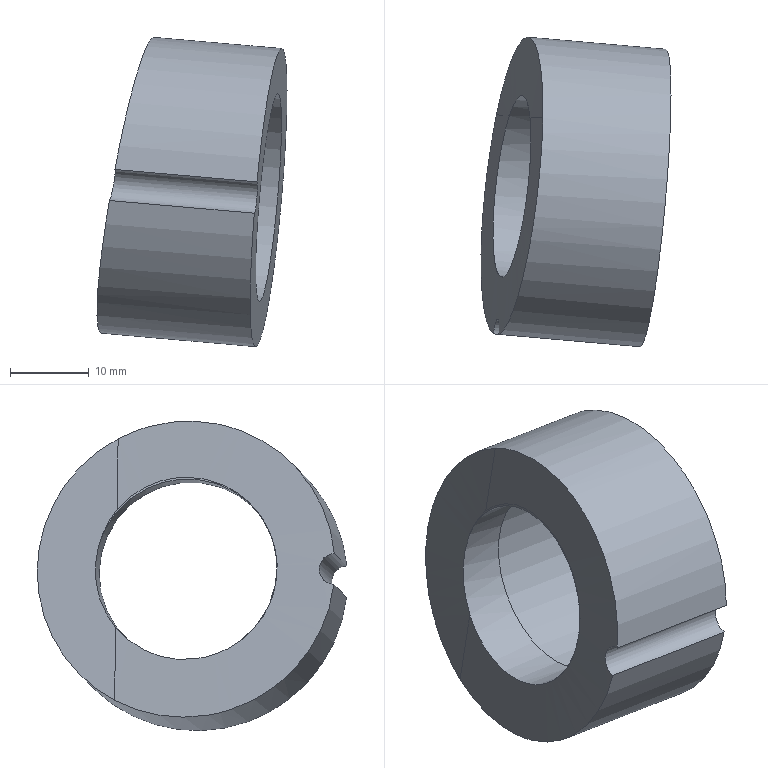Part | NX | features solid 2 | 1 solid | 10 faces | box 24.121 x 39.295 x 39.277 mm | volume 11087 mm3 | cylinder 4 | spline 4 | plane 2 | commonest cylinder face diameters 4 x1 23.2 x1 26.6 x1 38 x1
STEP:
#1=CARTESIAN_POINT('',(-929.483,-260.051,-35.553));
#2=VERTEX_POINT('',#1);
#3=CARTESIAN_POINT('',(-923.901,-232.605,-21.002));
#4=VERTEX_POINT('',#3);
#5=CARTESIAN_POINT('',(-929.483,-260.051,-35.553));
#6=CARTESIAN_POINT('',(-928.909,-259.773,-32.489));
#7=CARTESIAN_POINT('',(-927.663,-257.698,-26.623));
#8=CARTESIAN_POINT('',(-925.814,-250.756,-20.295));
#9=CARTESIAN_POINT('',(-924.374,-241.535,-18.016));
#10=CARTESIAN_POINT('',(-923.946,-235.373,-19.542));
#11=CARTESIAN_POINT('',(-923.901,-232.605,-21.002));
#12=B_SPLINE_CURVE_WITH_KNOTS('',3,(#5,#6,#7,#8,#9,#10,#11),.UNSPECIFIED.,.F.,.F.,(4,1,1,1,4),(0.,0.009255,0.01851,0.02776,0.03702),.UNSPECIFIED.);
#13=EDGE_CURVE('',#2,#4,#12,.T.);
#14=ORIENTED_EDGE('',*,*,#13,.F.);
#15=CARTESIAN_POINT('',(-911.448,-261.629,-37.137));
#16=VERTEX_POINT('',#15);
#17=CARTESIAN_POINT('',(-921.372,-260.761,-36.265));
#18=DIRECTION('',(-0.9924,0.08682,0.08716));
#19=VECTOR('',#18,1000.);
#20=LINE('',#17,#19);
#21=EDGE_CURVE('',#16,#2,#20,.T.);
#22=ORIENTED_EDGE('',*,*,#21,.F.);
#23=CARTESIAN_POINT('',(-911.795,-261.599,-41.116));
#24=VERTEX_POINT('',#23);
#25=CARTESIAN_POINT('',(-909.974,-242.791,-39.126));
#26=DIRECTION('',(-0.9924,0.08682,0.08716));
#27=DIRECTION('',(-0.08716,-0.9962,0.));
#28=AXIS2_PLACEMENT_3D('',#25,#26,#27);
#29=CIRCLE('',#28,19.);
#30=EDGE_CURVE('',#16,#24,#29,.T.);
#31=ORIENTED_EDGE('',*,*,#30,.T.);
#32=CARTESIAN_POINT('',(-930.183,-259.99,-39.501));
#33=VERTEX_POINT('',#32);
#34=CARTESIAN_POINT('',(-921.719,-260.731,-40.244));
#35=DIRECTION('',(-0.9924,0.08682,0.08716));
#36=VECTOR('',#35,1000.);
#37=LINE('',#34,#36);
#38=EDGE_CURVE('',#33,#24,#37,.F.);
#39=ORIENTED_EDGE('',*,*,#38,.F.);
#40=CARTESIAN_POINT('',(-929.786,-232.163,-54.19));
#41=VERTEX_POINT('',#40);
#42=CARTESIAN_POINT('',(-929.786,-232.163,-54.19));
#43=CARTESIAN_POINT('',(-930.342,-234.88,-55.62));
#44=CARTESIAN_POINT('',(-931.297,-240.963,-57.09));
#45=CARTESIAN_POINT('',(-931.921,-250.215,-54.784));
#46=CARTESIAN_POINT('',(-931.526,-257.369,-48.427));
#47=CARTESIAN_POINT('',(-930.693,-259.618,-42.557));
#48=CARTESIAN_POINT('',(-930.183,-259.99,-39.501));
#49=B_SPLINE_CURVE_WITH_KNOTS('',3,(#42,#43,#44,#45,#46,#47,#48),.UNSPECIFIED.,.F.,.F.,(4,1,1,1,4),(0.,0.00923,0.01846,0.02769,0.03692),.UNSPECIFIED.);
#50=EDGE_CURVE('',#41,#33,#49,.T.);
#51=ORIENTED_EDGE('',*,*,#50,.F.);
#52=CARTESIAN_POINT('',(-923.901,-232.605,-21.002));
#53=CARTESIAN_POINT('',(-923.851,-229.534,-22.621));
#54=CARTESIAN_POINT('',(-924.167,-224.375,-27.458));
#55=CARTESIAN_POINT('',(-925.684,-221.388,-37.657));
#56=CARTESIAN_POINT('',(-927.766,-224.091,-47.767));
#57=CARTESIAN_POINT('',(-929.167,-229.14,-52.598));
#58=CARTESIAN_POINT('',(-929.786,-232.163,-54.19));
#59=B_SPLINE_CURVE_WITH_KNOTS('',3,(#52,#53,#54,#55,#56,#57,#58),.UNSPECIFIED.,.F.,.F.,(4,1,1,1,4),(0.,0.01027,0.02053,0.0308,0.04107),.UNSPECIFIED.);
#60=EDGE_CURVE('',#4,#41,#59,.T.);
#61=ORIENTED_EDGE('',*,*,#60,.F.);
#62=EDGE_LOOP('',(#14,#22,#31,#39,#51,#61));
#63=FACE_BOUND('',#62,.T.);
#64=CARTESIAN_POINT('',(-909.974,-242.791,-39.126));
#65=DIRECTION('',(-0.9924,0.08682,0.08716));
#66=DIRECTION('',(-0.08716,-0.9962,0.));
#67=AXIS2_PLACEMENT_3D('',#64,#65,#66);
#68=CYLINDRICAL_SURFACE('',#67,19.);
#69=ADVANCED_FACE('',(#63),#68,.T.);
#70=CARTESIAN_POINT('',(-911.134,-256.041,-39.126));
#71=VERTEX_POINT('',#70);
#72=CARTESIAN_POINT('',(-909.974,-242.791,-39.126));
#73=DIRECTION('',(-0.9924,0.08682,0.08716));
#74=DIRECTION('',(-0.08716,-0.9962,0.));
#75=AXIS2_PLACEMENT_3D('',#72,#73,#74);
#76=CIRCLE('',#75,13.3);
#77=EDGE_CURVE('',#71,#71,#76,.T.);
#78=ORIENTED_EDGE('',*,*,#77,.T.);
#79=EDGE_LOOP('',(#78));
#80=FACE_BOUND('',#79,.T.);
#81=ORIENTED_EDGE('',*,*,#30,.F.);
#82=CARTESIAN_POINT('',(-911.63,-261.719,-39.126));
#83=DIRECTION('',(-0.9924,0.08682,0.08716));
#84=DIRECTION('',(-0.08716,-0.9962,0.));
#85=AXIS2_PLACEMENT_3D('',#82,#83,#84);
#86=CIRCLE('',#85,2.);
#87=EDGE_CURVE('',#16,#24,#86,.T.);
#88=ORIENTED_EDGE('',*,*,#87,.T.);
#89=EDGE_LOOP('',(#81,#88));
#90=FACE_BOUND('',#89,.T.);
#91=CARTESIAN_POINT('',(-909.974,-242.791,-39.126));
#92=DIRECTION('',(-0.9924,0.08682,0.08716));
#93=DIRECTION('',(-0.08716,-0.9962,0.));
#94=AXIS2_PLACEMENT_3D('',#91,#92,#93);
#95=PLANE('',#94);
#96=ADVANCED_FACE('',(#80,#90),#95,.F.);
#97=ORIENTED_EDGE('',*,*,#77,.F.);
#98=EDGE_LOOP('',(#97));
#99=FACE_BOUND('',#98,.T.);
#100=CARTESIAN_POINT('',(-923.042,-254.999,-38.08));
#101=VERTEX_POINT('',#100);
#102=CARTESIAN_POINT('',(-921.883,-241.749,-38.08));
#103=DIRECTION('',(-0.9924,0.08682,0.08716));
#104=DIRECTION('',(-0.08716,-0.9962,0.));
#105=AXIS2_PLACEMENT_3D('',#102,#103,#104);
#106=CIRCLE('',#105,13.3);
#107=EDGE_CURVE('',#101,#101,#106,.T.);
#108=ORIENTED_EDGE('',*,*,#107,.T.);
#109=EDGE_LOOP('',(#108));
#110=FACE_BOUND('',#109,.T.);
#111=CARTESIAN_POINT('',(-909.974,-242.791,-39.126));
#112=DIRECTION('',(-0.9924,0.08682,0.08716));
#113=DIRECTION('',(-0.08716,-0.9962,0.));
#114=AXIS2_PLACEMENT_3D('',#111,#112,#113);
#115=CYLINDRICAL_SURFACE('',#114,13.3);
#116=ADVANCED_FACE('',(#99,#110),#115,.F.);
#117=CARTESIAN_POINT('',(-922.894,-253.305,-38.08));
#118=VERTEX_POINT('',#117);
#119=CARTESIAN_POINT('',(-921.883,-241.749,-38.08));
#120=DIRECTION('',(-0.9924,0.08682,0.08716));
#121=DIRECTION('',(-0.08716,-0.9962,0.));
#122=AXIS2_PLACEMENT_3D('',#119,#120,#121);
#123=CIRCLE('',#122,11.6);
#124=EDGE_CURVE('',#118,#118,#123,.T.);
#125=ORIENTED_EDGE('',*,*,#124,.T.);
#126=EDGE_LOOP('',(#125));
#127=FACE_BOUND('',#126,.T.);
#128=ORIENTED_EDGE('',*,*,#107,.F.);
#129=EDGE_LOOP('',(#128));
#130=FACE_BOUND('',#129,.T.);
#131=CARTESIAN_POINT('',(-921.883,-241.749,-38.08));
#132=DIRECTION('',(-0.9924,0.08682,0.08716));
#133=DIRECTION('',(-0.08716,-0.9962,0.));
#134=AXIS2_PLACEMENT_3D('',#131,#132,#133);
#135=PLANE('',#134);
#136=ADVANCED_FACE('',(#127,#130),#135,.F.);
#137=ORIENTED_EDGE('',*,*,#21,.T.);
#138=CARTESIAN_POINT('',(-929.483,-260.051,-35.553));
#139=CARTESIAN_POINT('',(-929.439,-259.542,-35.58));
#140=CARTESIAN_POINT('',(-929.424,-258.559,-36.034));
#141=CARTESIAN_POINT('',(-929.629,-257.934,-37.53));
#142=CARTESIAN_POINT('',(-929.954,-258.513,-39.023));
#143=CARTESIAN_POINT('',(-930.129,-259.482,-39.475));
#144=CARTESIAN_POINT('',(-930.183,-259.99,-39.501));
#145=B_SPLINE_CURVE_WITH_KNOTS('',3,(#138,#139,#140,#141,#142,#143,#144),.UNSPECIFIED.,.F.,.F.,(4,1,1,1,4),(0.,0.001514,0.003028,0.004542,0.006057),.UNSPECIFIED.);
#146=EDGE_CURVE('',#2,#33,#145,.T.);
#147=ORIENTED_EDGE('',*,*,#146,.T.);
#148=ORIENTED_EDGE('',*,*,#38,.T.);
#149=ORIENTED_EDGE('',*,*,#87,.F.);
#150=EDGE_LOOP('',(#137,#147,#148,#149));
#151=FACE_BOUND('',#150,.T.);
#152=CARTESIAN_POINT('',(-911.63,-261.719,-39.126));
#153=DIRECTION('',(-0.9924,0.08682,0.08716));
#154=DIRECTION('',(-0.08716,-0.9962,0.));
#155=AXIS2_PLACEMENT_3D('',#152,#153,#154);
#156=CYLINDRICAL_SURFACE('',#155,2.);
#157=ADVANCED_FACE('',(#151),#156,.F.);
#158=CARTESIAN_POINT('',(-926.06,-230.143,-34.59));
#159=VERTEX_POINT('',#158);
#160=CARTESIAN_POINT('',(-925.539,-232.482,-30.239));
#161=VERTEX_POINT('',#160);
#162=CARTESIAN_POINT('',(-926.06,-230.143,-34.59));
#163=CARTESIAN_POINT('',(-925.828,-230.596,-33.013));
#164=CARTESIAN_POINT('',(-925.647,-231.395,-31.516));
#165=CARTESIAN_POINT('',(-925.539,-232.482,-30.239));
#166=B_SPLINE_CURVE_WITH_KNOTS('',3,(#162,#163,#164,#165),.UNSPECIFIED.,.F.,.F.,(4,4),(0.001876,0.006846),.UNSPECIFIED.);
#167=EDGE_CURVE('',#159,#161,#166,.T.);
#168=ORIENTED_EDGE('',*,*,#167,.F.);
#169=CARTESIAN_POINT('',(-928.148,-232.286,-44.953));
#170=VERTEX_POINT('',#169);
#171=CARTESIAN_POINT('',(-926.06,-230.143,-34.59));
#172=CARTESIAN_POINT('',(-926.584,-229.124,-38.139));
#173=CARTESIAN_POINT('',(-927.379,-229.926,-42.112));
#174=CARTESIAN_POINT('',(-928.148,-232.286,-44.953));
#175=B_SPLINE_CURVE_WITH_KNOTS('',3,(#171,#172,#173,#174),.UNSPECIFIED.,.F.,.F.,(4,4),(0.004979,0.01613),.UNSPECIFIED.);
#176=EDGE_CURVE('',#159,#170,#175,.T.);
#177=ORIENTED_EDGE('',*,*,#176,.T.);
#178=CARTESIAN_POINT('',(-930.229,-247.913,-46.785));
#179=VERTEX_POINT('',#178);
#180=CARTESIAN_POINT('',(-928.148,-232.286,-44.953));
#181=CARTESIAN_POINT('',(-928.747,-234.127,-47.168));
#182=CARTESIAN_POINT('',(-929.874,-239.507,-50.064));
#183=CARTESIAN_POINT('',(-930.275,-245.564,-48.485));
#184=CARTESIAN_POINT('',(-930.229,-247.913,-46.785));
#185=B_SPLINE_CURVE_WITH_KNOTS('',3,(#180,#181,#182,#183,#184),.UNSPECIFIED.,.F.,.F.,(4,1,4),(0.,0.0087,0.0174),.UNSPECIFIED.);
#186=EDGE_CURVE('',#170,#179,#185,.T.);
#187=ORIENTED_EDGE('',*,*,#186,.T.);
#188=CARTESIAN_POINT('',(-925.539,-232.482,-30.239));
#189=CARTESIAN_POINT('',(-925.326,-234.624,-27.725));
#190=CARTESIAN_POINT('',(-925.507,-241.044,-24.655));
#191=CARTESIAN_POINT('',(-927.325,-250.854,-28.707));
#192=CARTESIAN_POINT('',(-929.453,-254.13,-38.716));
#193=CARTESIAN_POINT('',(-930.177,-250.588,-44.848));
#194=CARTESIAN_POINT('',(-930.229,-247.913,-46.785));
#195=B_SPLINE_CURVE_WITH_KNOTS('',3,(#188,#189,#190,#191,#192,#193,#194),.UNSPECIFIED.,.F.,.F.,(4,1,1,1,4),(0.,0.009788,0.01958,0.02936,0.03915),.UNSPECIFIED.);
#196=EDGE_CURVE('',#161,#179,#195,.T.);
#197=ORIENTED_EDGE('',*,*,#196,.F.);
#198=EDGE_LOOP('',(#168,#177,#187,#197));
#199=FACE_BOUND('',#198,.T.);
#200=ORIENTED_EDGE('',*,*,#124,.F.);
#201=EDGE_LOOP('',(#200));
#202=FACE_BOUND('',#201,.T.);
#203=CARTESIAN_POINT('',(-909.974,-242.791,-39.126));
#204=DIRECTION('',(-0.9924,0.08682,0.08716));
#205=DIRECTION('',(-0.08716,-0.9962,0.));
#206=AXIS2_PLACEMENT_3D('',#203,#204,#205);
#207=CYLINDRICAL_SURFACE('',#206,11.6);
#208=ADVANCED_FACE('',(#199,#202),#207,.F.);
#209=CARTESIAN_POINT('',(-925.496,-232.485,-29.998));
#210=VERTEX_POINT('',#209);
#211=CARTESIAN_POINT('',(-925.496,-232.485,-29.998));
#212=CARTESIAN_POINT('',(-924.965,-232.525,-26.999));
#213=CARTESIAN_POINT('',(-924.433,-232.565,-24.001));
#214=CARTESIAN_POINT('',(-923.901,-232.605,-21.002));
#215=B_SPLINE_CURVE_WITH_KNOTS('',3,(#211,#212,#213,#214),.UNSPECIFIED.,.F.,.F.,(4,4),(0.,0.6033),.UNSPECIFIED.);
#216=EDGE_CURVE('',#210,#4,#215,.T.);
#217=ORIENTED_EDGE('',*,*,#216,.T.);
#218=ORIENTED_EDGE('',*,*,#60,.T.);
#219=CARTESIAN_POINT('',(-929.786,-232.163,-54.19));
#220=CARTESIAN_POINT('',(-929.24,-232.204,-51.111));
#221=CARTESIAN_POINT('',(-928.694,-232.245,-48.032));
#222=CARTESIAN_POINT('',(-928.148,-232.286,-44.953));
#223=B_SPLINE_CURVE_WITH_KNOTS('',3,(#219,#220,#221,#222),.UNSPECIFIED.,.F.,.F.,(4,4),(0.3603,0.9722),.UNSPECIFIED.);
#224=EDGE_CURVE('',#41,#170,#223,.T.);
#225=ORIENTED_EDGE('',*,*,#224,.T.);
#226=ORIENTED_EDGE('',*,*,#176,.F.);
#227=CARTESIAN_POINT('',(-926.06,-230.143,-34.59));
#228=CARTESIAN_POINT('',(-925.813,-230.555,-32.954));
#229=CARTESIAN_POINT('',(-925.613,-231.354,-31.348));
#230=CARTESIAN_POINT('',(-925.496,-232.485,-29.998));
#231=B_SPLINE_CURVE_WITH_KNOTS('',3,(#227,#228,#229,#230),.UNSPECIFIED.,.F.,.F.,(4,4),(0.6832,1.),.UNSPECIFIED.);
#232=EDGE_CURVE('',#159,#210,#231,.T.);
#233=ORIENTED_EDGE('',*,*,#232,.T.);
#234=EDGE_LOOP('',(#217,#218,#225,#226,#233));
#235=FACE_BOUND('',#234,.T.);
#236=CARTESIAN_POINT('',(-929.075,-221.938,-56.328));
#237=CARTESIAN_POINT('',(-923.118,-222.354,-22.742));
#238=CARTESIAN_POINT('',(-929.22,-223.985,-55.955));
#239=CARTESIAN_POINT('',(-923.263,-224.408,-22.369));
#240=CARTESIAN_POINT('',(-929.367,-226.031,-55.575));
#241=CARTESIAN_POINT('',(-923.41,-226.46,-21.989));
#242=CARTESIAN_POINT('',(-929.516,-228.076,-55.188));
#243=CARTESIAN_POINT('',(-923.56,-228.511,-21.602));
#244=CARTESIAN_POINT('',(-929.667,-230.119,-54.792));
#245=CARTESIAN_POINT('',(-923.712,-230.56,-21.206));
#246=CARTESIAN_POINT('',(-929.821,-232.16,-54.389));
#247=CARTESIAN_POINT('',(-923.866,-232.608,-20.803));
#248=B_SPLINE_SURFACE_WITH_KNOTS('',5,1,((#236,#237),(#238,#239),(#240,#241),(#242,#243),(#244,#245),(#246,#247)),.RULED_SURF.,.F.,.F.,.F.,(6,6),(2,2),(0.9701,1.),(0.1222,0.8673),.PIECEWISE_BEZIER_KNOTS.);
#249=ADVANCED_FACE('',(#235),#248,.T.);
#250=ORIENTED_EDGE('',*,*,#146,.F.);
#251=ORIENTED_EDGE('',*,*,#13,.T.);
#252=ORIENTED_EDGE('',*,*,#216,.F.);
#253=CARTESIAN_POINT('',(-925.752,-241.299,-25.884));
#254=VERTEX_POINT('',#253);
#255=CARTESIAN_POINT('',(-925.496,-232.485,-29.998));
#256=CARTESIAN_POINT('',(-925.439,-233.04,-29.336));
#257=CARTESIAN_POINT('',(-925.365,-234.254,-28.166));
#258=CARTESIAN_POINT('',(-925.384,-237.251,-26.392));
#259=CARTESIAN_POINT('',(-925.562,-239.62,-25.884));
#260=CARTESIAN_POINT('',(-925.752,-241.299,-25.884));
#261=B_SPLINE_CURVE_WITH_KNOTS('',3,(#255,#256,#257,#258,#259,#260),.UNSPECIFIED.,.F.,.F.,(4,1,1,4),(0.,0.25,0.5,1.),.UNSPECIFIED.);
#262=EDGE_CURVE('',#210,#254,#261,.T.);
#263=ORIENTED_EDGE('',*,*,#262,.T.);
#264=CARTESIAN_POINT('',(-929.986,-251.003,-43.546));
#265=VERTEX_POINT('',#264);
#266=CARTESIAN_POINT('',(-925.752,-241.299,-25.884));
#267=CARTESIAN_POINT('',(-925.983,-243.35,-25.883));
#268=CARTESIAN_POINT('',(-926.635,-247.369,-27.));
#269=CARTESIAN_POINT('',(-927.88,-251.708,-31.336));
#270=CARTESIAN_POINT('',(-928.941,-253.09,-36.457));
#271=CARTESIAN_POINT('',(-929.622,-252.482,-40.626));
#272=CARTESIAN_POINT('',(-929.886,-251.579,-42.64));
#273=CARTESIAN_POINT('',(-929.986,-251.003,-43.546));
#274=B_SPLINE_CURVE_WITH_KNOTS('',3,(#266,#267,#268,#269,#270,#271,#272,#273),.UNSPECIFIED.,.F.,.F.,(4,1,1,1,1,4),(0.,0.1726,0.3451,0.5177,0.604,0.6902),.UNSPECIFIED.);
#275=EDGE_CURVE('',#254,#265,#274,.T.);
#276=ORIENTED_EDGE('',*,*,#275,.T.);
#277=CARTESIAN_POINT('',(-929.986,-251.003,-43.546));
#278=CARTESIAN_POINT('',(-930.125,-250.206,-44.8));
#279=CARTESIAN_POINT('',(-930.21,-249.135,-45.925));
#280=CARTESIAN_POINT('',(-930.229,-247.913,-46.785));
#281=B_SPLINE_CURVE_WITH_KNOTS('',3,(#277,#278,#279,#280),.UNSPECIFIED.,.F.,.F.,(4,4),(0.6902,0.8097),.UNSPECIFIED.);
#282=EDGE_CURVE('',#265,#179,#281,.T.);
#283=ORIENTED_EDGE('',*,*,#282,.T.);
#284=ORIENTED_EDGE('',*,*,#186,.F.);
#285=ORIENTED_EDGE('',*,*,#224,.F.);
#286=ORIENTED_EDGE('',*,*,#50,.T.);
#287=EDGE_LOOP('',(#250,#251,#252,#263,#276,#283,#284,#285,#286));
#288=FACE_BOUND('',#287,.T.);
#289=CARTESIAN_POINT('',(-930.578,-232.103,-58.658));
#290=CARTESIAN_POINT('',(-923.705,-232.62,-19.898));
#291=CARTESIAN_POINT('',(-930.802,-235.077,-58.07));
#292=CARTESIAN_POINT('',(-923.93,-235.605,-19.31));
#293=CARTESIAN_POINT('',(-931.031,-238.047,-57.466));
#294=CARTESIAN_POINT('',(-924.159,-238.579,-18.706));
#295=CARTESIAN_POINT('',(-931.265,-241.031,-56.871));
#296=CARTESIAN_POINT('',(-924.394,-241.567,-18.11));
#297=CARTESIAN_POINT('',(-931.706,-246.571,-55.839));
#298=CARTESIAN_POINT('',(-924.836,-247.12,-17.079));
#299=CARTESIAN_POINT('',(-932.166,-252.147,-55.031));
#300=CARTESIAN_POINT('',(-925.298,-252.713,-16.27));
#301=CARTESIAN_POINT('',(-932.384,-254.74,-54.721));
#302=CARTESIAN_POINT('',(-925.515,-255.309,-15.961));
#303=CARTESIAN_POINT('',(-932.605,-257.336,-54.493));
#304=CARTESIAN_POINT('',(-925.738,-257.915,-15.733));
#305=CARTESIAN_POINT('',(-932.832,-259.934,-54.361));
#306=CARTESIAN_POINT('',(-925.965,-260.522,-15.601));
#307=B_SPLINE_SURFACE_WITH_KNOTS('',5,1,((#289,#290),(#291,#292),(#293,#294),(#295,#296),(#297,#298),(#299,#300),(#301,#302),(#303,#304),(#305,#306)),.RULED_SURF.,.F.,.F.,.F.,(6,3,6),(2,2),(0.,0.5001,0.9292),(0.02555,0.8074),.UNSPECIFIED.);
#308=ADVANCED_FACE('',(#288),#307,.T.);
#309=ORIENTED_EDGE('',*,*,#232,.F.);
#310=ORIENTED_EDGE('',*,*,#167,.T.);
#311=CARTESIAN_POINT('',(-925.496,-232.485,-29.998));
#312=CARTESIAN_POINT('',(-925.511,-232.484,-30.079));
#313=CARTESIAN_POINT('',(-925.525,-232.483,-30.159));
#314=CARTESIAN_POINT('',(-925.539,-232.482,-30.239));
#315=B_SPLINE_CURVE_WITH_KNOTS('',3,(#311,#312,#313,#314),.UNSPECIFIED.,.F.,.F.,(4,4),(0.,0.01658),.UNSPECIFIED.);
#316=EDGE_CURVE('',#161,#210,#315,.F.);
#317=ORIENTED_EDGE('',*,*,#316,.T.);
#318=EDGE_LOOP('',(#309,#310,#317));
#319=FACE_BOUND('',#318,.T.);
#320=CARTESIAN_POINT('',(-926.064,-230.129,-34.618));
#321=CARTESIAN_POINT('',(-925.32,-230.184,-30.423));
#322=CARTESIAN_POINT('',(-926.098,-230.589,-34.529));
#323=CARTESIAN_POINT('',(-925.354,-230.644,-30.334));
#324=CARTESIAN_POINT('',(-926.132,-231.049,-34.439));
#325=CARTESIAN_POINT('',(-925.388,-231.105,-30.244));
#326=CARTESIAN_POINT('',(-926.166,-231.51,-34.349));
#327=CARTESIAN_POINT('',(-925.423,-231.565,-30.154));
#328=CARTESIAN_POINT('',(-926.201,-231.97,-34.259));
#329=CARTESIAN_POINT('',(-925.457,-232.025,-30.064));
#330=CARTESIAN_POINT('',(-926.236,-232.43,-34.168));
#331=CARTESIAN_POINT('',(-925.492,-232.486,-29.973));
#332=B_SPLINE_SURFACE_WITH_KNOTS('',5,1,((#320,#321),(#322,#323),(#324,#325),(#326,#327),(#328,#329),(#330,#331)),.RULED_SURF.,.F.,.F.,.F.,(6,6),(2,2),(0.9933,1.),(0.5708,0.6638),.PIECEWISE_BEZIER_KNOTS.);
#333=ADVANCED_FACE('',(#319),#332,.T.);
#334=ORIENTED_EDGE('',*,*,#316,.F.);
#335=ORIENTED_EDGE('',*,*,#196,.T.);
#336=ORIENTED_EDGE('',*,*,#282,.F.);
#337=ORIENTED_EDGE('',*,*,#275,.F.);
#338=ORIENTED_EDGE('',*,*,#262,.F.);
#339=EDGE_LOOP('',(#334,#335,#336,#337,#338));
#340=FACE_BOUND('',#339,.T.);
#341=CARTESIAN_POINT('',(-929.021,-232.22,-49.878));
#342=CARTESIAN_POINT('',(-925.008,-232.522,-27.242));
#343=CARTESIAN_POINT('',(-929.245,-235.197,-49.291));
#344=CARTESIAN_POINT('',(-925.232,-235.505,-26.654));
#345=CARTESIAN_POINT('',(-929.474,-238.168,-48.687));
#346=CARTESIAN_POINT('',(-925.461,-238.478,-26.05));
#347=CARTESIAN_POINT('',(-929.708,-241.152,-48.091));
#348=CARTESIAN_POINT('',(-925.696,-241.466,-25.455));
#349=CARTESIAN_POINT('',(-930.036,-245.27,-47.325));
#350=CARTESIAN_POINT('',(-926.024,-245.589,-24.688));
#351=CARTESIAN_POINT('',(-930.375,-249.408,-46.681));
#352=CARTESIAN_POINT('',(-926.363,-249.733,-24.045));
#353=CARTESIAN_POINT('',(-930.469,-250.55,-46.515));
#354=CARTESIAN_POINT('',(-926.457,-250.877,-23.879));
#355=CARTESIAN_POINT('',(-930.564,-251.694,-46.361));
#356=CARTESIAN_POINT('',(-926.552,-252.023,-23.725));
#357=CARTESIAN_POINT('',(-930.66,-252.841,-46.22));
#358=CARTESIAN_POINT('',(-926.648,-253.171,-23.584));
#359=B_SPLINE_SURFACE_WITH_KNOTS('',5,1,((#341,#342),(#343,#344),(#345,#346),(#347,#348),(#349,#350),(#351,#352),(#353,#354),(#355,#356),(#357,#358)),.RULED_SURF.,.F.,.F.,.F.,(6,3,6),(2,2),(0.,0.5001,0.6903),(0.2026,0.6592),.UNSPECIFIED.);
#360=ADVANCED_FACE('',(#340),#359,.T.);
#361=CLOSED_SHELL('',(#69,#96,#116,#136,#157,#208,#249,#308,#333,#360));
#362=MANIFOLD_SOLID_BREP('',#361);
#363=(LENGTH_UNIT()NAMED_UNIT(*)SI_UNIT(.MILLI.,.METRE.));
#364=UNCERTAINTY_MEASURE_WITH_UNIT(LENGTH_MEASURE(0.05098),#363,'','');
#365=(NAMED_UNIT(*)PLANE_ANGLE_UNIT()SI_UNIT($,.RADIAN.));
#366=(NAMED_UNIT(*)SI_UNIT($,.STERADIAN.)SOLID_ANGLE_UNIT());
#367=(GEOMETRIC_REPRESENTATION_CONTEXT(3)GLOBAL_UNCERTAINTY_ASSIGNED_CONTEXT((#364))GLOBAL_UNIT_ASSIGNED_CONTEXT((#363,#365,#366))REPRESENTATION_CONTEXT('',''));
#368=ADVANCED_BREP_SHAPE_REPRESENTATION('',(#362),#367);